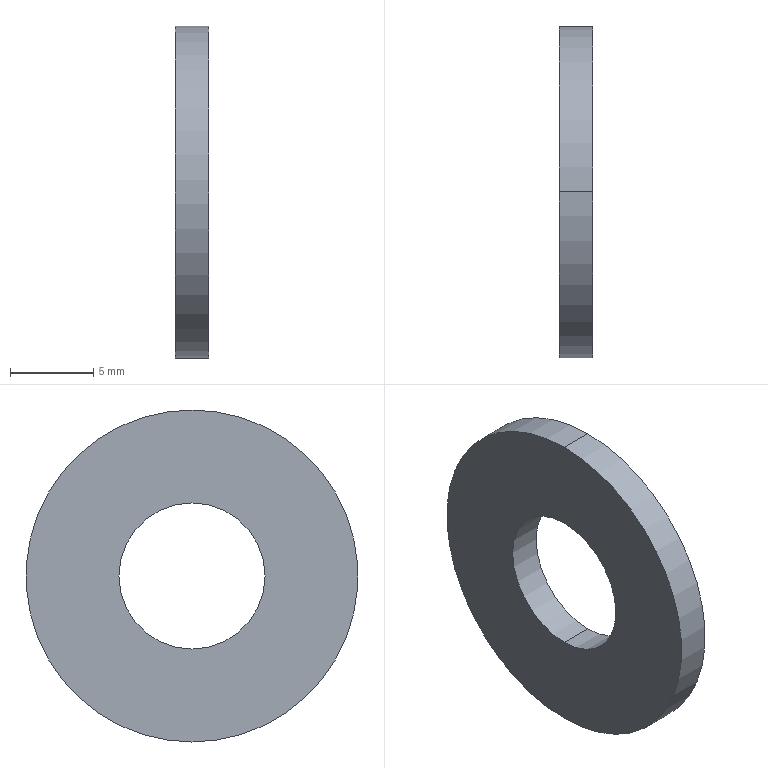Part | STEP file | plain washer 10669 type nl_iso_PreviewCfg | 1 solid | 6 faces | box 2 x 20 x 20 mm | volume 506.676 mm3 | cylinder 4 | plane 2 | commonest cylinder face diameters 8.8 x2 20 x2
STEP:
#1=CARTESIAN_POINT('',(0.,0.,0.));
#2=DIRECTION('',(0.,0.,1.));
#3=DIRECTION('',(1.,0.,0.));
#4=AXIS2_PLACEMENT_3D('',#1,#2,#3);
#5=CARTESIAN_POINT('',(2.,0.,4.4));
#6=VERTEX_POINT('',#5);
#7=CARTESIAN_POINT('',(0.,0.,4.4));
#8=VERTEX_POINT('',#7);
#9=CARTESIAN_POINT('',(2.,0.,4.4));
#10=DIRECTION('',(-1.,0.,0.));
#11=VECTOR('',#10,1.);
#12=LINE('',#9,#11);
#13=CARTESIAN_POINT('',(2.,0.,0.));
#14=DIRECTION('',(-1.,0.,0.));
#15=DIRECTION('',(0.,0.,1.));
#16=AXIS2_PLACEMENT_3D('',#13,#14,#15);
#17=CYLINDRICAL_SURFACE('',#16,4.4);
#18=CARTESIAN_POINT('',(6.283,0.));
#19=DIRECTION('',(0.,1.));
#20=VECTOR('',#19,1.);
#21=LINE('',#18,#20);
#22=(GEOMETRIC_REPRESENTATION_CONTEXT(2)PARAMETRIC_REPRESENTATION_CONTEXT()REPRESENTATION_CONTEXT('',''));
#23=DEFINITIONAL_REPRESENTATION('',(#21),#22);
#24=PCURVE('',#17,#23);
#25=CARTESIAN_POINT('',(2.,0.,0.));
#26=DIRECTION('',(-1.,0.,0.));
#27=DIRECTION('',(0.,0.,1.));
#28=AXIS2_PLACEMENT_3D('',#25,#26,#27);
#29=CYLINDRICAL_SURFACE('',#28,4.4);
#30=CARTESIAN_POINT('',(0.,0.));
#31=DIRECTION('',(0.,1.));
#32=VECTOR('',#31,1.);
#33=LINE('',#30,#32);
#34=(GEOMETRIC_REPRESENTATION_CONTEXT(2)PARAMETRIC_REPRESENTATION_CONTEXT()REPRESENTATION_CONTEXT('',''));
#35=DEFINITIONAL_REPRESENTATION('',(#33),#34);
#36=PCURVE('',#29,#35);
#37=SURFACE_CURVE('',#12,(#24,#36),.PCURVE_S1.);
#38=EDGE_CURVE('',#6,#8,#37,.T.);
#39=ORIENTED_EDGE('',*,*,#38,.T.);
#40=CARTESIAN_POINT('',(0.,0.,-4.4));
#41=VERTEX_POINT('',#40);
#42=CARTESIAN_POINT('',(0.,0.,0.));
#43=DIRECTION('',(1.,0.,0.));
#44=DIRECTION('',(0.,0.,-1.));
#45=AXIS2_PLACEMENT_3D('',#42,#43,#44);
#46=CIRCLE('',#45,4.4);
#47=CARTESIAN_POINT('',(9.425,2.));
#48=DIRECTION('',(-1.,0.));
#49=VECTOR('',#48,1.);
#50=LINE('',#47,#49);
#51=(GEOMETRIC_REPRESENTATION_CONTEXT(2)PARAMETRIC_REPRESENTATION_CONTEXT()REPRESENTATION_CONTEXT('',''));
#52=DEFINITIONAL_REPRESENTATION('',(#50),#51);
#53=PCURVE('',#17,#52);
#54=CARTESIAN_POINT('',(0.,0.,0.));
#55=DIRECTION('',(1.,0.,0.));
#56=DIRECTION('',(0.,0.,-1.));
#57=AXIS2_PLACEMENT_3D('',#54,#55,#56);
#58=PLANE('',#57);
#59=CARTESIAN_POINT('',(0.,0.));
#60=DIRECTION('',(1.,0.));
#61=AXIS2_PLACEMENT_2D('',#59,#60);
#62=CIRCLE('',#61,4.4);
#63=(GEOMETRIC_REPRESENTATION_CONTEXT(2)PARAMETRIC_REPRESENTATION_CONTEXT()REPRESENTATION_CONTEXT('',''));
#64=DEFINITIONAL_REPRESENTATION('',(#62),#63);
#65=PCURVE('',#58,#64);
#66=SURFACE_CURVE('',#46,(#53,#65),.PCURVE_S1.);
#67=EDGE_CURVE('',#8,#41,#66,.T.);
#68=ORIENTED_EDGE('',*,*,#67,.T.);
#69=CARTESIAN_POINT('',(2.,0.,-4.4));
#70=VERTEX_POINT('',#69);
#71=CARTESIAN_POINT('',(2.,0.,-4.4));
#72=DIRECTION('',(-1.,0.,0.));
#73=VECTOR('',#72,1.);
#74=LINE('',#71,#73);
#75=CARTESIAN_POINT('',(3.142,0.));
#76=DIRECTION('',(0.,1.));
#77=VECTOR('',#76,1.);
#78=LINE('',#75,#77);
#79=(GEOMETRIC_REPRESENTATION_CONTEXT(2)PARAMETRIC_REPRESENTATION_CONTEXT()REPRESENTATION_CONTEXT('',''));
#80=DEFINITIONAL_REPRESENTATION('',(#78),#79);
#81=PCURVE('',#17,#80);
#82=CARTESIAN_POINT('',(3.142,0.));
#83=DIRECTION('',(0.,1.));
#84=VECTOR('',#83,1.);
#85=LINE('',#82,#84);
#86=(GEOMETRIC_REPRESENTATION_CONTEXT(2)PARAMETRIC_REPRESENTATION_CONTEXT()REPRESENTATION_CONTEXT('',''));
#87=DEFINITIONAL_REPRESENTATION('',(#85),#86);
#88=PCURVE('',#29,#87);
#89=SURFACE_CURVE('',#74,(#81,#88),.PCURVE_S1.);
#90=EDGE_CURVE('',#70,#41,#89,.T.);
#91=ORIENTED_EDGE('',*,*,#90,.F.);
#92=CARTESIAN_POINT('',(2.,0.,0.));
#93=DIRECTION('',(1.,0.,0.));
#94=DIRECTION('',(0.,0.,-1.));
#95=AXIS2_PLACEMENT_3D('',#92,#93,#94);
#96=CIRCLE('',#95,4.4);
#97=CARTESIAN_POINT('',(9.425,0.));
#98=DIRECTION('',(-1.,0.));
#99=VECTOR('',#98,1.);
#100=LINE('',#97,#99);
#101=(GEOMETRIC_REPRESENTATION_CONTEXT(2)PARAMETRIC_REPRESENTATION_CONTEXT()REPRESENTATION_CONTEXT('',''));
#102=DEFINITIONAL_REPRESENTATION('',(#100),#101);
#103=PCURVE('',#17,#102);
#104=CARTESIAN_POINT('',(2.,0.,0.));
#105=DIRECTION('',(1.,0.,0.));
#106=DIRECTION('',(0.,0.,-1.));
#107=AXIS2_PLACEMENT_3D('',#104,#105,#106);
#108=PLANE('',#107);
#109=CARTESIAN_POINT('',(0.,0.));
#110=DIRECTION('',(1.,0.));
#111=AXIS2_PLACEMENT_2D('',#109,#110);
#112=CIRCLE('',#111,4.4);
#113=(GEOMETRIC_REPRESENTATION_CONTEXT(2)PARAMETRIC_REPRESENTATION_CONTEXT()REPRESENTATION_CONTEXT('',''));
#114=DEFINITIONAL_REPRESENTATION('',(#112),#113);
#115=PCURVE('',#108,#114);
#116=SURFACE_CURVE('',#96,(#103,#115),.PCURVE_S1.);
#117=EDGE_CURVE('',#6,#70,#116,.T.);
#118=ORIENTED_EDGE('',*,*,#117,.F.);
#119=EDGE_LOOP('',(#39,#68,#91,#118));
#120=FACE_BOUND('',#119,.F.);
#121=ADVANCED_FACE('',(#120),#17,.F.);
#122=CARTESIAN_POINT('',(2.,0.,-10.));
#123=VERTEX_POINT('',#122);
#124=CARTESIAN_POINT('',(2.,0.,10.));
#125=VERTEX_POINT('',#124);
#126=CARTESIAN_POINT('',(2.,0.,0.));
#127=DIRECTION('',(1.,0.,0.));
#128=DIRECTION('',(0.,0.,-1.));
#129=AXIS2_PLACEMENT_3D('',#126,#127,#128);
#130=CIRCLE('',#129,10.);
#131=CARTESIAN_POINT('',(2.,0.,0.));
#132=DIRECTION('',(-1.,0.,0.));
#133=DIRECTION('',(0.,0.,1.));
#134=AXIS2_PLACEMENT_3D('',#131,#132,#133);
#135=CYLINDRICAL_SURFACE('',#134,10.);
#136=CARTESIAN_POINT('',(3.142,0.));
#137=DIRECTION('',(-1.,0.));
#138=VECTOR('',#137,1.);
#139=LINE('',#136,#138);
#140=(GEOMETRIC_REPRESENTATION_CONTEXT(2)PARAMETRIC_REPRESENTATION_CONTEXT()REPRESENTATION_CONTEXT('',''));
#141=DEFINITIONAL_REPRESENTATION('',(#139),#140);
#142=PCURVE('',#135,#141);
#143=CARTESIAN_POINT('',(0.,0.));
#144=DIRECTION('',(1.,0.));
#145=AXIS2_PLACEMENT_2D('',#143,#144);
#146=CIRCLE('',#145,10.);
#147=(GEOMETRIC_REPRESENTATION_CONTEXT(2)PARAMETRIC_REPRESENTATION_CONTEXT()REPRESENTATION_CONTEXT('',''));
#148=DEFINITIONAL_REPRESENTATION('',(#146),#147);
#149=PCURVE('',#108,#148);
#150=SURFACE_CURVE('',#130,(#142,#149),.PCURVE_S1.);
#151=EDGE_CURVE('',#123,#125,#150,.T.);
#152=ORIENTED_EDGE('',*,*,#151,.F.);
#153=CARTESIAN_POINT('',(0.,0.,-10.));
#154=VERTEX_POINT('',#153);
#155=CARTESIAN_POINT('',(2.,0.,-10.));
#156=DIRECTION('',(-1.,0.,0.));
#157=VECTOR('',#156,1.);
#158=LINE('',#155,#157);
#159=CARTESIAN_POINT('',(3.142,0.));
#160=DIRECTION('',(0.,1.));
#161=VECTOR('',#160,1.);
#162=LINE('',#159,#161);
#163=(GEOMETRIC_REPRESENTATION_CONTEXT(2)PARAMETRIC_REPRESENTATION_CONTEXT()REPRESENTATION_CONTEXT('',''));
#164=DEFINITIONAL_REPRESENTATION('',(#162),#163);
#165=PCURVE('',#135,#164);
#166=CARTESIAN_POINT('',(2.,0.,0.));
#167=DIRECTION('',(-1.,0.,0.));
#168=DIRECTION('',(0.,0.,1.));
#169=AXIS2_PLACEMENT_3D('',#166,#167,#168);
#170=CYLINDRICAL_SURFACE('',#169,10.);
#171=CARTESIAN_POINT('',(3.142,0.));
#172=DIRECTION('',(0.,1.));
#173=VECTOR('',#172,1.);
#174=LINE('',#171,#173);
#175=(GEOMETRIC_REPRESENTATION_CONTEXT(2)PARAMETRIC_REPRESENTATION_CONTEXT()REPRESENTATION_CONTEXT('',''));
#176=DEFINITIONAL_REPRESENTATION('',(#174),#175);
#177=PCURVE('',#170,#176);
#178=SURFACE_CURVE('',#158,(#165,#177),.PCURVE_S1.);
#179=EDGE_CURVE('',#123,#154,#178,.T.);
#180=ORIENTED_EDGE('',*,*,#179,.T.);
#181=CARTESIAN_POINT('',(0.,0.,10.));
#182=VERTEX_POINT('',#181);
#183=CARTESIAN_POINT('',(0.,0.,0.));
#184=DIRECTION('',(1.,0.,0.));
#185=DIRECTION('',(0.,0.,-1.));
#186=AXIS2_PLACEMENT_3D('',#183,#184,#185);
#187=CIRCLE('',#186,10.);
#188=CARTESIAN_POINT('',(3.142,2.));
#189=DIRECTION('',(-1.,0.));
#190=VECTOR('',#189,1.);
#191=LINE('',#188,#190);
#192=(GEOMETRIC_REPRESENTATION_CONTEXT(2)PARAMETRIC_REPRESENTATION_CONTEXT()REPRESENTATION_CONTEXT('',''));
#193=DEFINITIONAL_REPRESENTATION('',(#191),#192);
#194=PCURVE('',#135,#193);
#195=CARTESIAN_POINT('',(0.,0.));
#196=DIRECTION('',(1.,0.));
#197=AXIS2_PLACEMENT_2D('',#195,#196);
#198=CIRCLE('',#197,10.);
#199=(GEOMETRIC_REPRESENTATION_CONTEXT(2)PARAMETRIC_REPRESENTATION_CONTEXT()REPRESENTATION_CONTEXT('',''));
#200=DEFINITIONAL_REPRESENTATION('',(#198),#199);
#201=PCURVE('',#58,#200);
#202=SURFACE_CURVE('',#187,(#194,#201),.PCURVE_S1.);
#203=EDGE_CURVE('',#154,#182,#202,.T.);
#204=ORIENTED_EDGE('',*,*,#203,.T.);
#205=CARTESIAN_POINT('',(2.,0.,10.));
#206=DIRECTION('',(-1.,0.,0.));
#207=VECTOR('',#206,1.);
#208=LINE('',#205,#207);
#209=CARTESIAN_POINT('',(0.,0.));
#210=DIRECTION('',(0.,1.));
#211=VECTOR('',#210,1.);
#212=LINE('',#209,#211);
#213=(GEOMETRIC_REPRESENTATION_CONTEXT(2)PARAMETRIC_REPRESENTATION_CONTEXT()REPRESENTATION_CONTEXT('',''));
#214=DEFINITIONAL_REPRESENTATION('',(#212),#213);
#215=PCURVE('',#135,#214);
#216=CARTESIAN_POINT('',(6.283,0.));
#217=DIRECTION('',(0.,1.));
#218=VECTOR('',#217,1.);
#219=LINE('',#216,#218);
#220=(GEOMETRIC_REPRESENTATION_CONTEXT(2)PARAMETRIC_REPRESENTATION_CONTEXT()REPRESENTATION_CONTEXT('',''));
#221=DEFINITIONAL_REPRESENTATION('',(#219),#220);
#222=PCURVE('',#170,#221);
#223=SURFACE_CURVE('',#208,(#215,#222),.PCURVE_S1.);
#224=EDGE_CURVE('',#125,#182,#223,.T.);
#225=ORIENTED_EDGE('',*,*,#224,.F.);
#226=EDGE_LOOP('',(#152,#180,#204,#225));
#227=FACE_BOUND('',#226,.T.);
#228=ADVANCED_FACE('',(#227),#135,.T.);
#229=CARTESIAN_POINT('',(2.,0.,0.));
#230=DIRECTION('',(1.,0.,0.));
#231=DIRECTION('',(0.,0.,-1.));
#232=AXIS2_PLACEMENT_3D('',#229,#230,#231);
#233=CIRCLE('',#232,10.);
#234=CARTESIAN_POINT('',(0.,0.));
#235=DIRECTION('',(1.,0.));
#236=AXIS2_PLACEMENT_2D('',#234,#235);
#237=CIRCLE('',#236,10.);
#238=(GEOMETRIC_REPRESENTATION_CONTEXT(2)PARAMETRIC_REPRESENTATION_CONTEXT()REPRESENTATION_CONTEXT('',''));
#239=DEFINITIONAL_REPRESENTATION('',(#237),#238);
#240=PCURVE('',#108,#239);
#241=CARTESIAN_POINT('',(9.425,0.));
#242=DIRECTION('',(-1.,0.));
#243=VECTOR('',#242,1.);
#244=LINE('',#241,#243);
#245=(GEOMETRIC_REPRESENTATION_CONTEXT(2)PARAMETRIC_REPRESENTATION_CONTEXT()REPRESENTATION_CONTEXT('',''));
#246=DEFINITIONAL_REPRESENTATION('',(#244),#245);
#247=PCURVE('',#170,#246);
#248=SURFACE_CURVE('',#233,(#240,#247),.PCURVE_S1.);
#249=EDGE_CURVE('',#125,#123,#248,.T.);
#250=ORIENTED_EDGE('',*,*,#249,.T.);
#251=ORIENTED_EDGE('',*,*,#151,.T.);
#252=EDGE_LOOP('',(#250,#251));
#253=FACE_BOUND('',#252,.T.);
#254=ORIENTED_EDGE('',*,*,#117,.F.);
#255=CARTESIAN_POINT('',(2.,0.,0.));
#256=DIRECTION('',(1.,0.,0.));
#257=DIRECTION('',(0.,0.,-1.));
#258=AXIS2_PLACEMENT_3D('',#255,#256,#257);
#259=CIRCLE('',#258,4.4);
#260=CARTESIAN_POINT('',(0.,0.));
#261=DIRECTION('',(1.,0.));
#262=AXIS2_PLACEMENT_2D('',#260,#261);
#263=CIRCLE('',#262,4.4);
#264=(GEOMETRIC_REPRESENTATION_CONTEXT(2)PARAMETRIC_REPRESENTATION_CONTEXT()REPRESENTATION_CONTEXT('',''));
#265=DEFINITIONAL_REPRESENTATION('',(#263),#264);
#266=PCURVE('',#108,#265);
#267=CARTESIAN_POINT('',(3.142,0.));
#268=DIRECTION('',(-1.,0.));
#269=VECTOR('',#268,1.);
#270=LINE('',#267,#269);
#271=(GEOMETRIC_REPRESENTATION_CONTEXT(2)PARAMETRIC_REPRESENTATION_CONTEXT()REPRESENTATION_CONTEXT('',''));
#272=DEFINITIONAL_REPRESENTATION('',(#270),#271);
#273=PCURVE('',#29,#272);
#274=SURFACE_CURVE('',#259,(#266,#273),.PCURVE_S1.);
#275=EDGE_CURVE('',#70,#6,#274,.T.);
#276=ORIENTED_EDGE('',*,*,#275,.F.);
#277=EDGE_LOOP('',(#254,#276));
#278=FACE_BOUND('',#277,.T.);
#279=ADVANCED_FACE('',(#253,#278),#108,.T.);
#280=CARTESIAN_POINT('',(0.,0.,0.));
#281=DIRECTION('',(1.,0.,0.));
#282=DIRECTION('',(0.,0.,-1.));
#283=AXIS2_PLACEMENT_3D('',#280,#281,#282);
#284=CIRCLE('',#283,10.);
#285=CARTESIAN_POINT('',(0.,0.));
#286=DIRECTION('',(1.,0.));
#287=AXIS2_PLACEMENT_2D('',#285,#286);
#288=CIRCLE('',#287,10.);
#289=(GEOMETRIC_REPRESENTATION_CONTEXT(2)PARAMETRIC_REPRESENTATION_CONTEXT()REPRESENTATION_CONTEXT('',''));
#290=DEFINITIONAL_REPRESENTATION('',(#288),#289);
#291=PCURVE('',#58,#290);
#292=CARTESIAN_POINT('',(9.425,2.));
#293=DIRECTION('',(-1.,0.));
#294=VECTOR('',#293,1.);
#295=LINE('',#292,#294);
#296=(GEOMETRIC_REPRESENTATION_CONTEXT(2)PARAMETRIC_REPRESENTATION_CONTEXT()REPRESENTATION_CONTEXT('',''));
#297=DEFINITIONAL_REPRESENTATION('',(#295),#296);
#298=PCURVE('',#170,#297);
#299=SURFACE_CURVE('',#284,(#291,#298),.PCURVE_S1.);
#300=EDGE_CURVE('',#182,#154,#299,.T.);
#301=ORIENTED_EDGE('',*,*,#300,.F.);
#302=ORIENTED_EDGE('',*,*,#203,.F.);
#303=EDGE_LOOP('',(#301,#302));
#304=FACE_BOUND('',#303,.T.);
#305=ORIENTED_EDGE('',*,*,#67,.T.);
#306=CARTESIAN_POINT('',(0.,0.,0.));
#307=DIRECTION('',(1.,0.,0.));
#308=DIRECTION('',(0.,0.,-1.));
#309=AXIS2_PLACEMENT_3D('',#306,#307,#308);
#310=CIRCLE('',#309,4.4);
#311=CARTESIAN_POINT('',(0.,0.));
#312=DIRECTION('',(1.,0.));
#313=AXIS2_PLACEMENT_2D('',#311,#312);
#314=CIRCLE('',#313,4.4);
#315=(GEOMETRIC_REPRESENTATION_CONTEXT(2)PARAMETRIC_REPRESENTATION_CONTEXT()REPRESENTATION_CONTEXT('',''));
#316=DEFINITIONAL_REPRESENTATION('',(#314),#315);
#317=PCURVE('',#58,#316);
#318=CARTESIAN_POINT('',(3.142,2.));
#319=DIRECTION('',(-1.,0.));
#320=VECTOR('',#319,1.);
#321=LINE('',#318,#320);
#322=(GEOMETRIC_REPRESENTATION_CONTEXT(2)PARAMETRIC_REPRESENTATION_CONTEXT()REPRESENTATION_CONTEXT('',''));
#323=DEFINITIONAL_REPRESENTATION('',(#321),#322);
#324=PCURVE('',#29,#323);
#325=SURFACE_CURVE('',#310,(#317,#324),.PCURVE_S1.);
#326=EDGE_CURVE('',#41,#8,#325,.T.);
#327=ORIENTED_EDGE('',*,*,#326,.T.);
#328=EDGE_LOOP('',(#305,#327));
#329=FACE_BOUND('',#328,.T.);
#330=ADVANCED_FACE('',(#304,#329),#58,.F.);
#331=ORIENTED_EDGE('',*,*,#179,.F.);
#332=ORIENTED_EDGE('',*,*,#249,.F.);
#333=ORIENTED_EDGE('',*,*,#224,.T.);
#334=ORIENTED_EDGE('',*,*,#300,.T.);
#335=EDGE_LOOP('',(#331,#332,#333,#334));
#336=FACE_BOUND('',#335,.T.);
#337=ADVANCED_FACE('',(#336),#170,.T.);
#338=ORIENTED_EDGE('',*,*,#326,.T.);
#339=ORIENTED_EDGE('',*,*,#38,.F.);
#340=ORIENTED_EDGE('',*,*,#275,.F.);
#341=ORIENTED_EDGE('',*,*,#90,.T.);
#342=EDGE_LOOP('',(#338,#339,#340,#341));
#343=FACE_BOUND('',#342,.F.);
#344=ADVANCED_FACE('',(#343),#29,.F.);
#345=CLOSED_SHELL('',(#121,#228,#279,#330,#337,#344));
#346=MANIFOLD_SOLID_BREP('',#345);
#347=(LENGTH_UNIT()NAMED_UNIT(*)SI_UNIT(.MILLI.,.METRE.));
#348=UNCERTAINTY_MEASURE_WITH_UNIT(LENGTH_MEASURE(0.0000001),#347,'','');
#349=(NAMED_UNIT(*)PLANE_ANGLE_UNIT()SI_UNIT($,.RADIAN.));
#350=(NAMED_UNIT(*)SI_UNIT($,.STERADIAN.)SOLID_ANGLE_UNIT());
#351=(GEOMETRIC_REPRESENTATION_CONTEXT(3)GLOBAL_UNCERTAINTY_ASSIGNED_CONTEXT((#348))GLOBAL_UNIT_ASSIGNED_CONTEXT((#347,#349,#350))REPRESENTATION_CONTEXT('',''));
#352=ADVANCED_BREP_SHAPE_REPRESENTATION('',(#4,#346),#351);